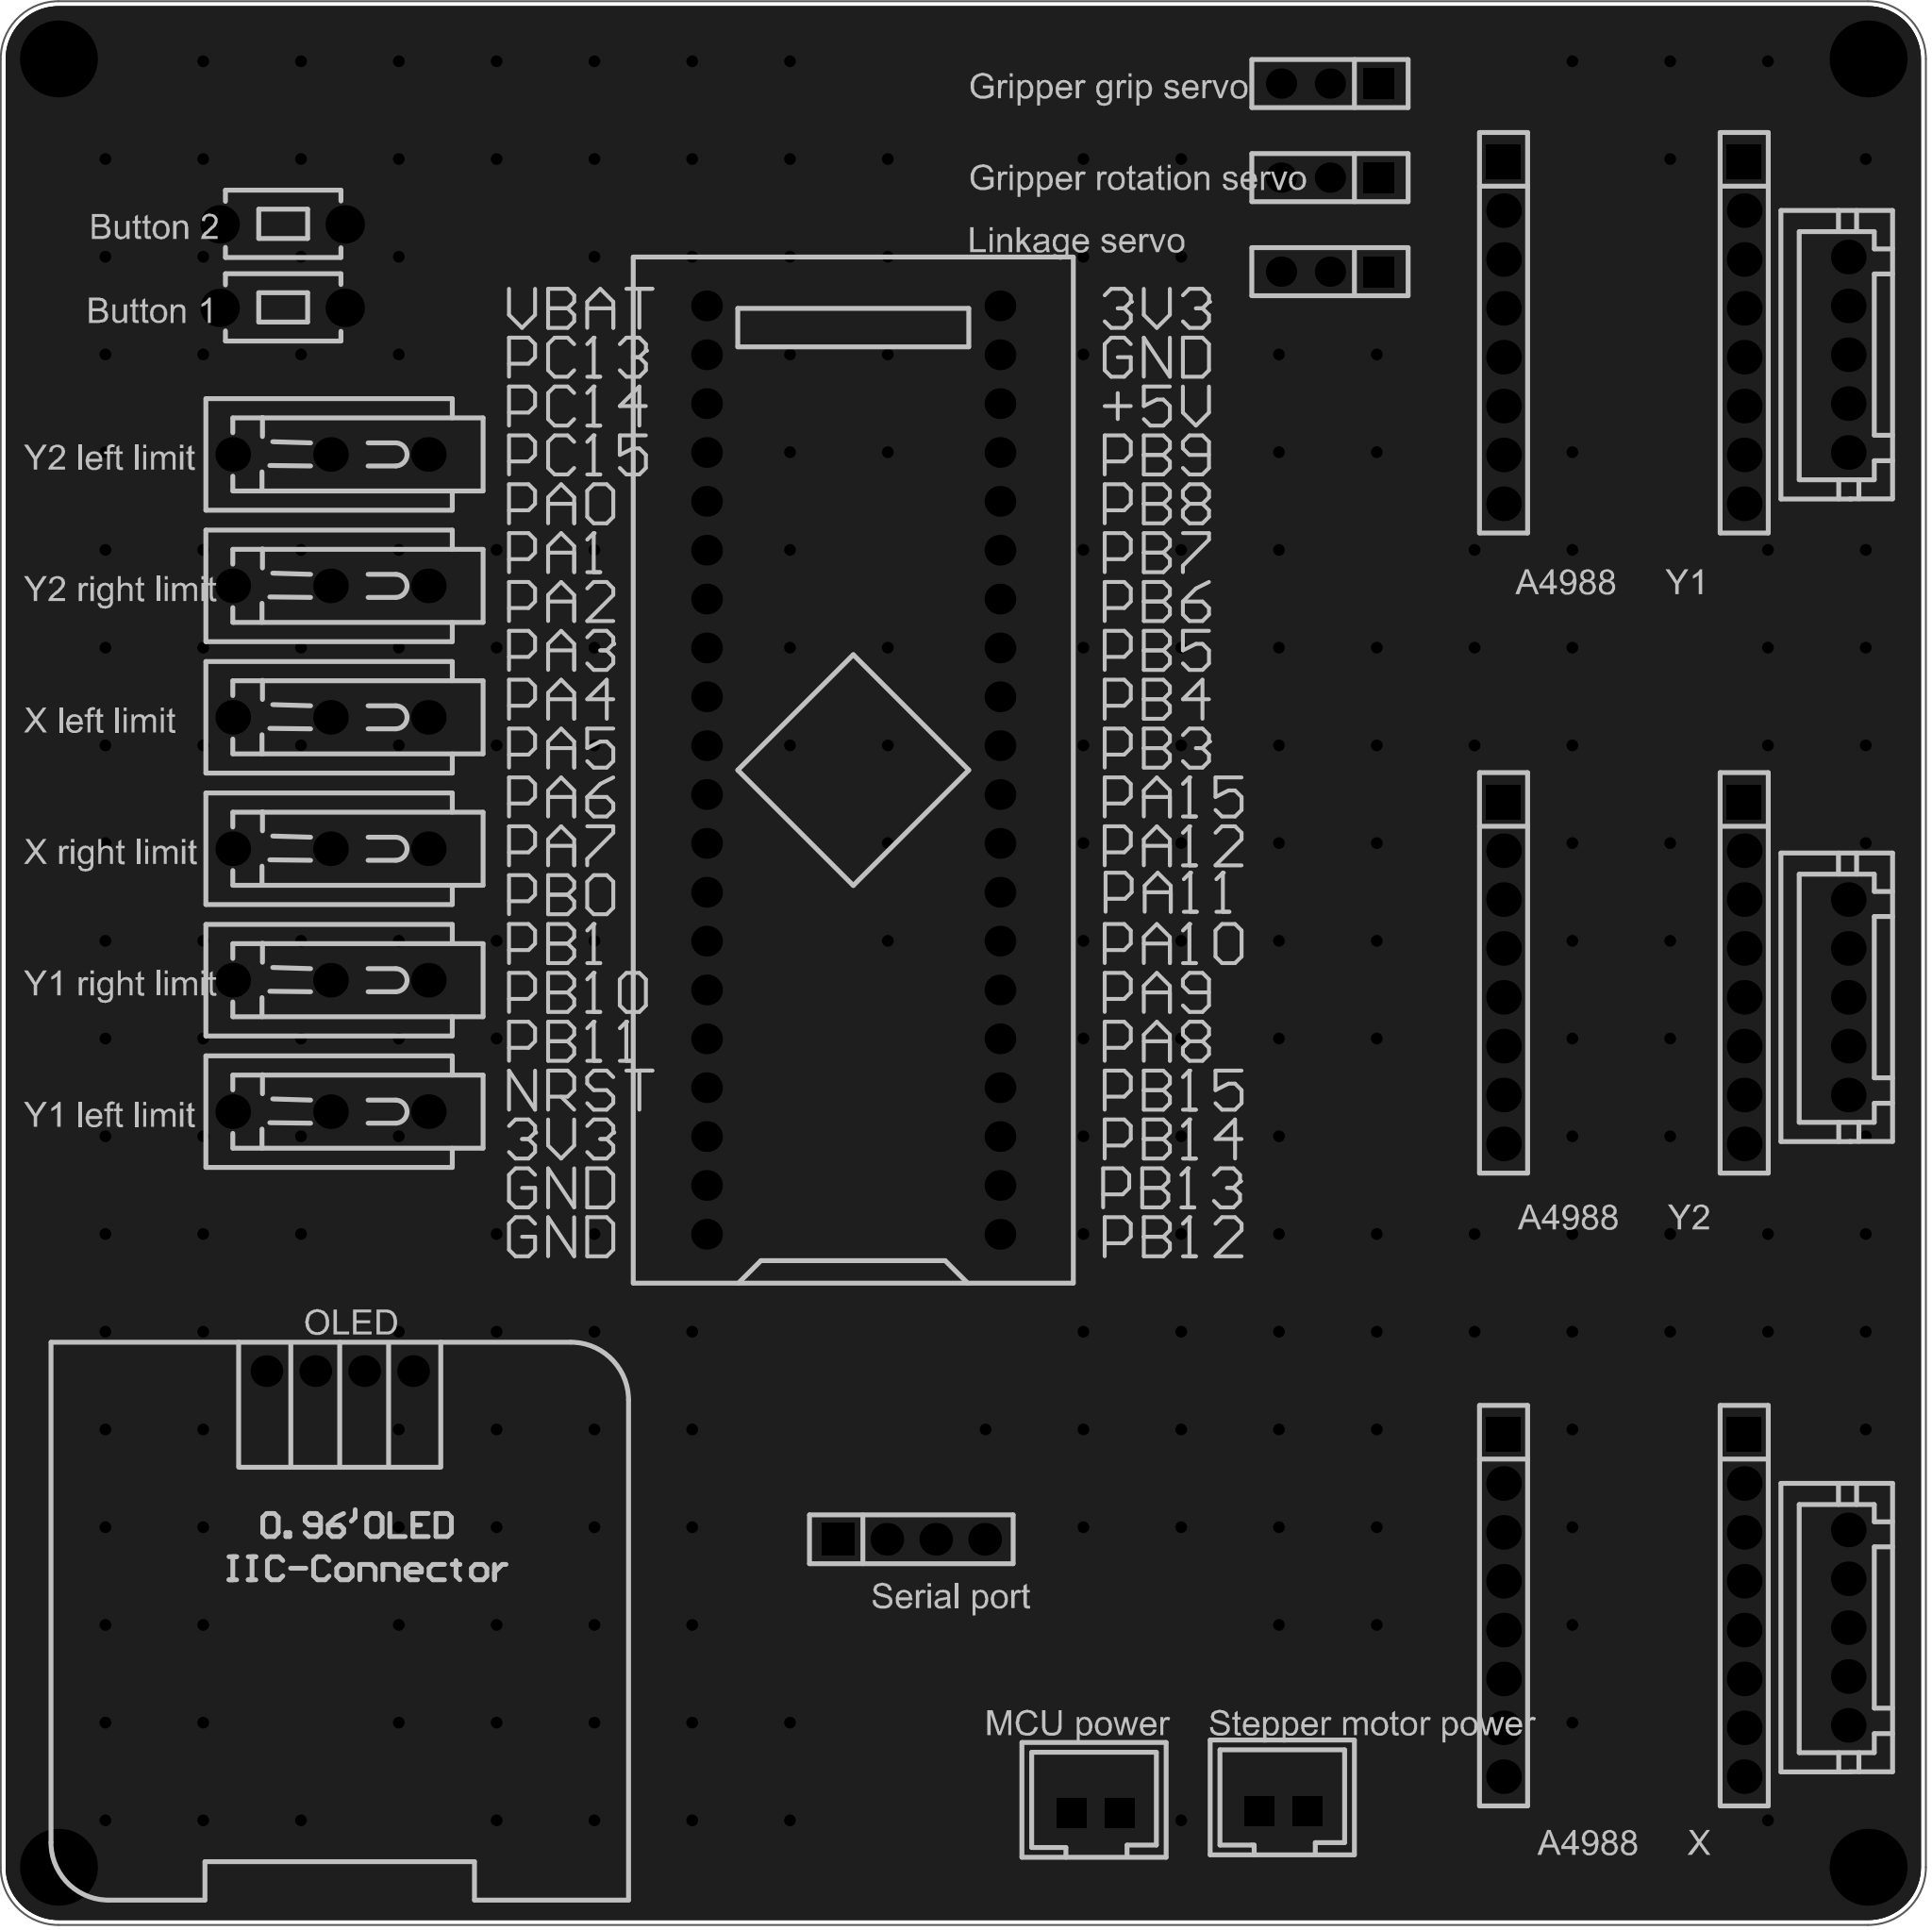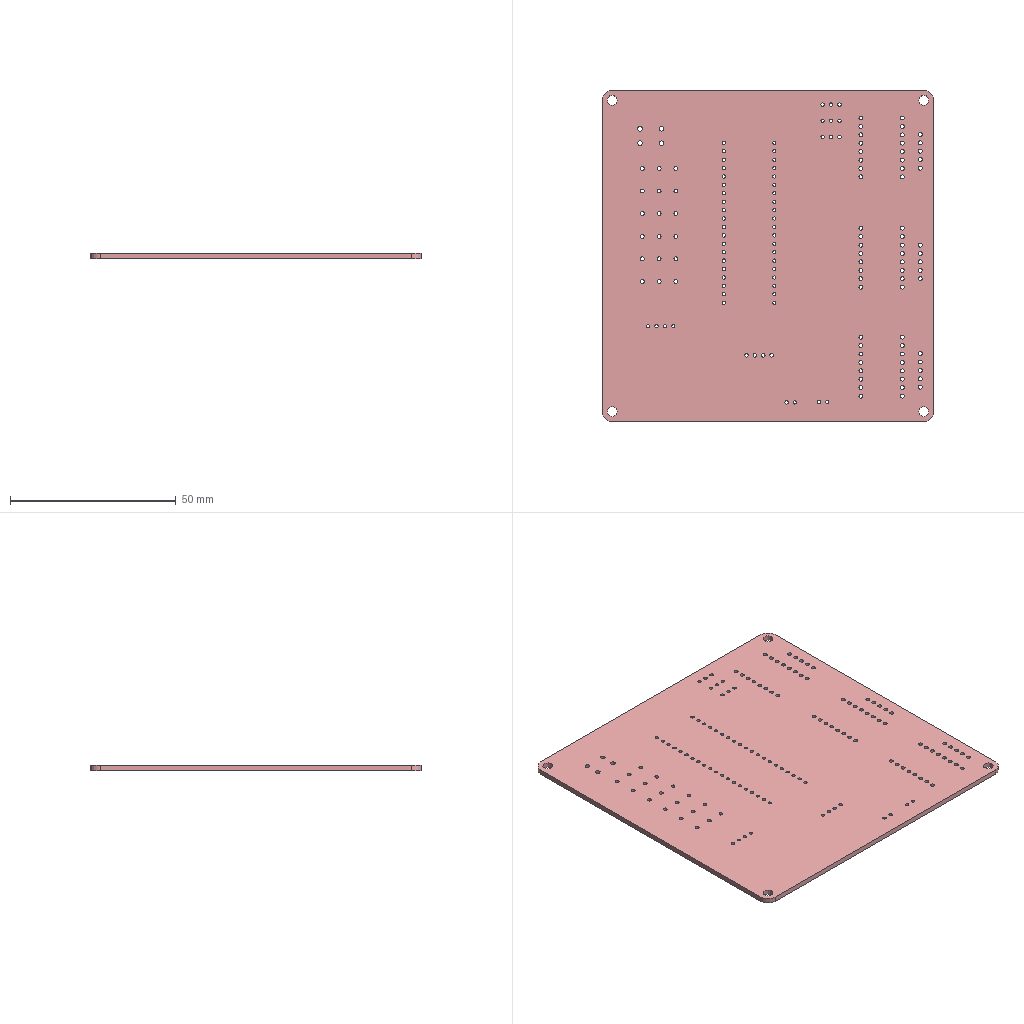Circuit board layout | Altium Designer | box 100 x 100 x 1.6 mm
Layer stack:
# Altium Designer layer stack of  (unit mm; dielectric type: 0 none, 1 core, 2 prepreg, 3 surface material)
index,name,kind,layer,copper_thickness_mm,dielectric_type,dielectric_thickness_mm,dielectric_material,dielectric_constant
0,Top Paste Mask Layer,other,,,,,,
1,Top Silkscreen Layer,other,,,,,,
2,Top Solder Mask Layer,dielectric,,,3,0.01,,3.3
3,Top Layer,copper,Top Layer,0.035,,,,
4,Dielectric1,dielectric,,,3,1.51,FR4,4.5
5,Bottom Layer,copper,Bottom Layer,0.035,,,,
6,Bottom Solder Mask Layer,dielectric,,,3,0.01,,3.3
7,Bottom Silkscreen Layer,other,,,,,,
8,Bottom Paste Mask Layer,other,,,,,,
# drill layer pairs: low layer,high layer
drill_pair,Top Layer,Bottom Layer
Part placement:
Designator,Comment,Layer,Footprint,Center-X(mm),Center-Y(mm),Rotation
U1,STM32F103C8T6-Card,TopLayer,CONN-TH_L53.3-W22.9_STM32F103C8T6-CARD,135.636,143.256,90
OLED1,,TopLayer,0.96OLED_4P,108.962,112.014,0
CN1,XH2.54-5P,TopLayer,CONN-TH_5P-P2.54_C9900008095,187.321,164.846,270
CN2,XH2.54-5P,TopLayer,CONN-TH_5P-P2.54_C9900008095,187.321,131.445,270
CN4,XH2.54-2PIN-straight pin,TopLayer,CONN-TH_XH2.54-2P,157.984,89.154,0
H1,,TopLayer,HDR-TH_8P-P2.54-V-F-1,169.414,165.989,270
H2,,TopLayer,HDR-TH_8P-P2.54-V-F-1,181.914,165.989,270
H3,,TopLayer,HDR-TH_4P-P2.54-V-F,138.651,103.272,0
SW6,3JWD-DBHD-13.5 125,TopLayer,SW-TH_SHOU-HAN_3JWD-DBHD-13.5,108.483,145.999,0
H4,,TopLayer,HDR-TH_8P-P2.54-V-F-1,169.414,132.715,270
CN3,XH2.54-5P,TopLayer,CONN-TH_5P-P2.54_C9900008095,187.321,98.679,270
H5,,TopLayer,HDR-TH_8P-P2.54-V-F-1,181.914,132.715,270
SW7,3JWD-DBHD-13.5 125,TopLayer,SW-TH_SHOU-HAN_3JWD-DBHD-13.5,108.483,152.832,0
H6,,TopLayer,HDR-TH_8P-P2.54-V-F-1,169.414,99.822,270
SW3,3JWD-DBHD-13.5 125,TopLayer,SW-TH_SHOU-HAN_3JWD-DBHD-13.5,108.483,125.501,0
SW8,3JWD-DBHD-13.5 125,TopLayer,SW-TH_SHOU-HAN_3JWD-DBHD-13.5,108.483,159.664,0
H8,,TopLayer,HDR-TH_3P-P2.54-V-F,160.397,174.054,180
H9,,TopLayer,HDR-TH_3P-P2.54-V-F,160.397,178.943,180
SW1,,TopLayer,Key_TH_3.5x6x4.3,105.974,171.623,180
H10,,TopLayer,HDR-TH_3P-P2.54-V-F,160.397,169.164,180
SW2,,TopLayer,Key_TH_3.5x6x4.3,105.974,167.28,180
SW4,3JWD-DBHD-13.5 125,TopLayer,SW-TH_SHOU-HAN_3JWD-DBHD-13.5,108.483,132.334,0
SW5,3JWD-DBHD-13.5 125,TopLayer,SW-TH_SHOU-HAN_3JWD-DBHD-13.5,108.483,139.167,0
H7,,TopLayer,HDR-TH_8P-P2.54-V-F-1,181.914,99.822,270
CN5,XH2.54-2PIN-straight pin,TopLayer,CONN-TH_XH2.54-2P,148.205,89.027,0
Pad and via stacks:
# Altium Designer via and pad stacks of  (unit mm). Each distinct definition once, with the count of objects using it.
# via: kind,start_layer,end_layer,hole_mm,diameter_mm,mode(0 simple;1 top-mid-bottom;2 full stack),diameter_per_layer,count,example_net
# pad: kind,layer,hole_mm,hole_type(0 round;1 square;2 slot),plating,top_size,top_shape(1 round;2 rect;3 octagon;9 rounded rect),mid_size,bottom_size,mode,footprint,size_per_layer,count,example
pad,Multi-Layer,3,0,plated,4x4,1,4x4,4x4,0,,,4,1
pad,Multi-Layer,1,0,plated,1.6x1.6,1,1.6x1.6,1.6x1.6,0,CONN-TH_L53.3-W22.9_STM32F103C8T6-CARD,,40,U1.1
pad,Multi-Layer,1,0,plated,1.65x1.65,1,1.65x1.65,1.65x1.65,0,0.96OLED_4P,,4,OLED1.4
pad,Multi-Layer,1.2,0,plated,1.8x1.8,1,1.8x1.8,1.8x1.8,0,CONN-TH_5P-P2.54_C9900008095,,15,CN1.5
pad,Multi-Layer,1,2,plated,1.524x1.524,2,1.524x1.524,1.524x1.524,0,CONN-TH_XH2.54-2P,,4,CN4.1
pad,Multi-Layer,1.2,0,plated,1.8x1.8,2,1.8x1.8,1.8x1.8,0,HDR-TH_8P-P2.54-V-F-1,,6,H1.1
pad,Multi-Layer,1.2,0,plated,1.8x1.8,1,1.8x1.8,1.8x1.8,0,HDR-TH_8P-P2.54-V-F-1,,42,H1.2
pad,Multi-Layer,1.1,0,plated,1.7x1.7,2,1.7x1.7,1.7x1.7,0,HDR-TH_4P-P2.54-V-F,,1,H3.1
pad,Multi-Layer,1.1,0,plated,1.7x1.7,1,1.7x1.7,1.7x1.7,0,HDR-TH_4P-P2.54-V-F,,3,H3.2
pad,Multi-Layer,1.2,0,plated,1.8x1.8,1,1.8x1.8,1.8x1.8,0,SW-TH_SHOU-HAN_3JWD-DBHD-13.5,,18,SW6.1
pad,Multi-Layer,1.02,0,plated,1.575x1.575,1,1.575x1.575,1.575x1.575,0,HDR-TH_3P-P2.54-V-F,,6,H8.3
pad,Multi-Layer,1.02,0,plated,1.575x1.575,2,1.575x1.575,1.575x1.575,0,HDR-TH_3P-P2.54-V-F,,3,H8.1
pad,Multi-Layer,1.399,0,plated,1.999x1.999,1,1.999x1.999,1.999x1.999,0,Key_TH_3.5x6x4.3,,4,SW1.A
via,Top Layer,Bottom Layer,0.3048,0.61,0,,216,GND
Copper pours:
name,layer,net,type(0 solid;1 hatched;2 none)
Bottom Layer-GND,Bottom Layer,GND,0
Top Layer-GND,Top Layer,GND,0
Top Layer-GND 1,Top Layer,GND,0
Design rules, without the lines most boards share:
# Altium Designer design rules of  (exported by Altium Designer, unit mm)
# columns: name | kind | enabled | priority | scope1 | scope2 | descriptor | typed fields (field=value)
Copper_copperRegion_copperThickness1oz | 0 | disabled | 4 | All | All | Clearance Constraint (Gap=5.984mil) (Disabled)(All),(All) | gap=0.152
Copper_copperRegion_copperThickness1oz_1 | 63 | disabled | 4 | All | All | Board Clearance Constraint (Gap=0mil) (Disabled)(All) |
Copper_copperRegion_Copper_copperRegion | 0 | disabled | 5 | All | All | Clearance Constraint (Gap=5.984mil) (Disabled)(All),(All) | gap=0.152
Copper_copperRegion_Copper_copperRegion_1 | 63 | disabled | 5 | All | All | Board Clearance Constraint (Gap=0mil) (Disabled)(All) |
copperThickness1oz | 0 | enabled | 6 | All | All | Clearance Constraint (Gap=5.984mil) (All),(All) | gap=0.152
copperThickness1oz_1 | 63 | enabled | 6 | All | All | Board Clearance Constraint (Gap=0mil) (All) |
copperRegion_copperThickness1oz | 20 | disabled | 1 | All | All | Polygon Connect Rule(Relief Connect )(Conductor Width=10mil) (Relief Angle=90 Angle) (Entries=4) (Air Gap Width=10mil) (Disabled)(All),(All) | connect_style(0=relief,1=direct,2=none)=0 relief_conductor_width=0.254 relief_entries=4
copperRegion_Copper_copperRegion | 20 | disabled | 2 | All | All | Polygon Connect Rule(Relief Connect )(Conductor Width=10mil) (Relief Angle=90 Angle) (Entries=4) (Air Gap Width=10mil) (Disabled)(All),(All) | connect_style(0=relief,1=direct,2=none)=0 relief_conductor_width=0.254 relief_entries=4
copperRegion | 20 | enabled | 3 | All | All | Polygon Connect Rule(Relief Connect )(Conductor Width=10mil) (Relief Angle=90 Angle) (Entries=4) (Air Gap Width=10mil) (All),(All) | connect_style(0=relief,1=direct,2=none)=0 relief_conductor_width=0.254 relief_entries=4